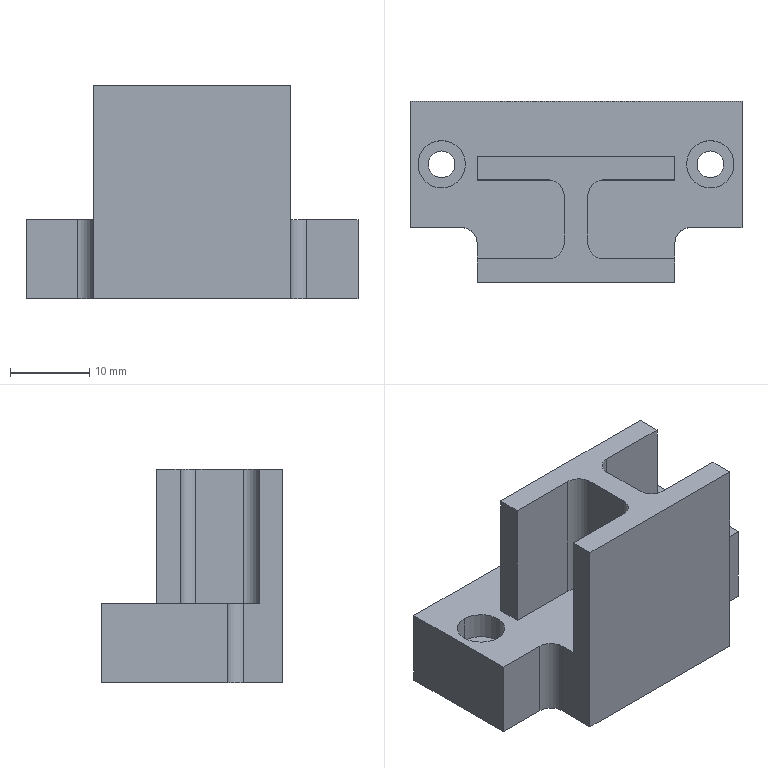Part | NX | 1 solid | 36 faces | box 42 x 23 x 27 mm | volume 11293 mm3 | plane 22 | cylinder 14 | commonest cylinder face diameters 4 x6 3.4 x4 6 x4
STEP:
#1=CARTESIAN_POINT('',(17.,6.5,-20.4));
#2=VERTEX_POINT('',#1);
#3=CARTESIAN_POINT('',(17.,0.5,-20.4));
#4=VERTEX_POINT('',#3);
#5=CARTESIAN_POINT('',(17.,3.5,-20.4));
#6=DIRECTION('',(0.,0.,1.));
#7=DIRECTION('',(0.,-1.,0.));
#8=AXIS2_PLACEMENT_3D('',#5,#6,#7);
#9=CIRCLE('',#8,3.);
#10=EDGE_CURVE('',#2,#4,#9,.T.);
#11=ORIENTED_EDGE('',*,*,#10,.F.);
#12=CARTESIAN_POINT('',(17.,6.5,-17.));
#13=VERTEX_POINT('',#12);
#14=CARTESIAN_POINT('',(17.,6.5,-17.));
#15=DIRECTION('',(0.,0.,1.));
#16=VECTOR('',#15,1000.);
#17=LINE('',#14,#16);
#18=EDGE_CURVE('',#13,#2,#17,.F.);
#19=ORIENTED_EDGE('',*,*,#18,.F.);
#20=CARTESIAN_POINT('',(17.,0.5,-17.));
#21=VERTEX_POINT('',#20);
#22=CARTESIAN_POINT('',(17.,3.5,-17.));
#23=DIRECTION('',(0.,0.,1.));
#24=DIRECTION('',(0.,-1.,0.));
#25=AXIS2_PLACEMENT_3D('',#22,#23,#24);
#26=CIRCLE('',#25,3.);
#27=EDGE_CURVE('',#13,#21,#26,.T.);
#28=ORIENTED_EDGE('',*,*,#27,.T.);
#29=CARTESIAN_POINT('',(17.,0.5,-17.));
#30=DIRECTION('',(0.,0.,1.));
#31=VECTOR('',#30,1000.);
#32=LINE('',#29,#31);
#33=EDGE_CURVE('',#21,#4,#32,.F.);
#34=ORIENTED_EDGE('',*,*,#33,.T.);
#35=EDGE_LOOP('',(#11,#19,#28,#34));
#36=FACE_BOUND('',#35,.T.);
#37=CARTESIAN_POINT('',(17.,3.5,-17.));
#38=DIRECTION('',(0.,0.,1.));
#39=DIRECTION('',(0.,1.,0.));
#40=AXIS2_PLACEMENT_3D('',#37,#38,#39);
#41=CYLINDRICAL_SURFACE('',#40,3.);
#42=ADVANCED_FACE('',(#36),#41,.F.);
#43=CARTESIAN_POINT('',(17.,5.2,-27.));
#44=VERTEX_POINT('',#43);
#45=CARTESIAN_POINT('',(17.,1.8,-27.));
#46=VERTEX_POINT('',#45);
#47=CARTESIAN_POINT('',(17.,3.5,-27.));
#48=DIRECTION('',(0.,0.,1.));
#49=DIRECTION('',(0.,-1.,0.));
#50=AXIS2_PLACEMENT_3D('',#47,#48,#49);
#51=CIRCLE('',#50,1.7);
#52=EDGE_CURVE('',#44,#46,#51,.T.);
#53=ORIENTED_EDGE('',*,*,#52,.F.);
#54=CARTESIAN_POINT('',(17.,5.2,-20.4));
#55=VERTEX_POINT('',#54);
#56=CARTESIAN_POINT('',(17.,5.2,-17.));
#57=DIRECTION('',(0.,0.,1.));
#58=VECTOR('',#57,1000.);
#59=LINE('',#56,#58);
#60=EDGE_CURVE('',#55,#44,#59,.F.);
#61=ORIENTED_EDGE('',*,*,#60,.F.);
#62=CARTESIAN_POINT('',(17.,1.8,-20.4));
#63=VERTEX_POINT('',#62);
#64=CARTESIAN_POINT('',(17.,3.5,-20.4));
#65=DIRECTION('',(0.,0.,1.));
#66=DIRECTION('',(0.,-1.,0.));
#67=AXIS2_PLACEMENT_3D('',#64,#65,#66);
#68=CIRCLE('',#67,1.7);
#69=EDGE_CURVE('',#55,#63,#68,.T.);
#70=ORIENTED_EDGE('',*,*,#69,.T.);
#71=CARTESIAN_POINT('',(17.,1.8,-17.));
#72=DIRECTION('',(0.,0.,1.));
#73=VECTOR('',#72,1000.);
#74=LINE('',#71,#73);
#75=EDGE_CURVE('',#63,#46,#74,.F.);
#76=ORIENTED_EDGE('',*,*,#75,.T.);
#77=EDGE_LOOP('',(#53,#61,#70,#76));
#78=FACE_BOUND('',#77,.T.);
#79=CARTESIAN_POINT('',(17.,3.5,-17.));
#80=DIRECTION('',(0.,0.,1.));
#81=DIRECTION('',(0.,1.,0.));
#82=AXIS2_PLACEMENT_3D('',#79,#80,#81);
#83=CYLINDRICAL_SURFACE('',#82,1.7);
#84=ADVANCED_FACE('',(#78),#83,.F.);
#85=CARTESIAN_POINT('',(-17.,6.5,-20.4));
#86=VERTEX_POINT('',#85);
#87=CARTESIAN_POINT('',(-17.,0.5,-20.4));
#88=VERTEX_POINT('',#87);
#89=CARTESIAN_POINT('',(-17.,3.5,-20.4));
#90=DIRECTION('',(0.,0.,1.));
#91=DIRECTION('',(0.,-1.,0.));
#92=AXIS2_PLACEMENT_3D('',#89,#90,#91);
#93=CIRCLE('',#92,3.);
#94=EDGE_CURVE('',#86,#88,#93,.T.);
#95=ORIENTED_EDGE('',*,*,#94,.F.);
#96=CARTESIAN_POINT('',(-17.,6.5,-17.));
#97=VERTEX_POINT('',#96);
#98=CARTESIAN_POINT('',(-17.,6.5,-17.));
#99=DIRECTION('',(0.,0.,1.));
#100=VECTOR('',#99,1000.);
#101=LINE('',#98,#100);
#102=EDGE_CURVE('',#97,#86,#101,.F.);
#103=ORIENTED_EDGE('',*,*,#102,.F.);
#104=CARTESIAN_POINT('',(-17.,0.5,-17.));
#105=VERTEX_POINT('',#104);
#106=CARTESIAN_POINT('',(-17.,3.5,-17.));
#107=DIRECTION('',(0.,0.,1.));
#108=DIRECTION('',(0.,-1.,0.));
#109=AXIS2_PLACEMENT_3D('',#106,#107,#108);
#110=CIRCLE('',#109,3.);
#111=EDGE_CURVE('',#97,#105,#110,.T.);
#112=ORIENTED_EDGE('',*,*,#111,.T.);
#113=CARTESIAN_POINT('',(-17.,0.5,-17.));
#114=DIRECTION('',(0.,0.,1.));
#115=VECTOR('',#114,1000.);
#116=LINE('',#113,#115);
#117=EDGE_CURVE('',#105,#88,#116,.F.);
#118=ORIENTED_EDGE('',*,*,#117,.T.);
#119=EDGE_LOOP('',(#95,#103,#112,#118));
#120=FACE_BOUND('',#119,.T.);
#121=CARTESIAN_POINT('',(-17.,3.5,-17.));
#122=DIRECTION('',(0.,0.,1.));
#123=DIRECTION('',(0.,1.,0.));
#124=AXIS2_PLACEMENT_3D('',#121,#122,#123);
#125=CYLINDRICAL_SURFACE('',#124,3.);
#126=ADVANCED_FACE('',(#120),#125,.F.);
#127=CARTESIAN_POINT('',(-17.,5.2,-27.));
#128=VERTEX_POINT('',#127);
#129=CARTESIAN_POINT('',(-17.,1.8,-27.));
#130=VERTEX_POINT('',#129);
#131=CARTESIAN_POINT('',(-17.,3.5,-27.));
#132=DIRECTION('',(0.,0.,1.));
#133=DIRECTION('',(0.,-1.,0.));
#134=AXIS2_PLACEMENT_3D('',#131,#132,#133);
#135=CIRCLE('',#134,1.7);
#136=EDGE_CURVE('',#128,#130,#135,.T.);
#137=ORIENTED_EDGE('',*,*,#136,.F.);
#138=CARTESIAN_POINT('',(-17.,5.2,-20.4));
#139=VERTEX_POINT('',#138);
#140=CARTESIAN_POINT('',(-17.,5.2,-17.));
#141=DIRECTION('',(0.,0.,1.));
#142=VECTOR('',#141,1000.);
#143=LINE('',#140,#142);
#144=EDGE_CURVE('',#139,#128,#143,.F.);
#145=ORIENTED_EDGE('',*,*,#144,.F.);
#146=CARTESIAN_POINT('',(-17.,1.8,-20.4));
#147=VERTEX_POINT('',#146);
#148=CARTESIAN_POINT('',(-17.,3.5,-20.4));
#149=DIRECTION('',(0.,0.,1.));
#150=DIRECTION('',(0.,-1.,0.));
#151=AXIS2_PLACEMENT_3D('',#148,#149,#150);
#152=CIRCLE('',#151,1.7);
#153=EDGE_CURVE('',#139,#147,#152,.T.);
#154=ORIENTED_EDGE('',*,*,#153,.T.);
#155=CARTESIAN_POINT('',(-17.,1.8,-17.));
#156=DIRECTION('',(0.,0.,1.));
#157=VECTOR('',#156,1000.);
#158=LINE('',#155,#157);
#159=EDGE_CURVE('',#147,#130,#158,.F.);
#160=ORIENTED_EDGE('',*,*,#159,.T.);
#161=EDGE_LOOP('',(#137,#145,#154,#160));
#162=FACE_BOUND('',#161,.T.);
#163=CARTESIAN_POINT('',(-17.,3.5,-17.));
#164=DIRECTION('',(0.,0.,1.));
#165=DIRECTION('',(0.,1.,0.));
#166=AXIS2_PLACEMENT_3D('',#163,#164,#165);
#167=CYLINDRICAL_SURFACE('',#166,1.7);
#168=ADVANCED_FACE('',(#162),#167,.F.);
#169=CARTESIAN_POINT('',(-17.,3.5,-17.));
#170=DIRECTION('',(0.,0.,1.));
#171=DIRECTION('',(0.,-1.,0.));
#172=AXIS2_PLACEMENT_3D('',#169,#170,#171);
#173=CIRCLE('',#172,3.);
#174=EDGE_CURVE('',#105,#97,#173,.T.);
#175=ORIENTED_EDGE('',*,*,#174,.F.);
#176=ORIENTED_EDGE('',*,*,#111,.F.);
#177=EDGE_LOOP('',(#175,#176));
#178=FACE_BOUND('',#177,.T.);
#179=CARTESIAN_POINT('',(17.,3.5,-17.));
#180=DIRECTION('',(0.,0.,1.));
#181=DIRECTION('',(0.,-1.,0.));
#182=AXIS2_PLACEMENT_3D('',#179,#180,#181);
#183=CIRCLE('',#182,3.);
#184=EDGE_CURVE('',#21,#13,#183,.T.);
#185=ORIENTED_EDGE('',*,*,#184,.F.);
#186=ORIENTED_EDGE('',*,*,#27,.F.);
#187=EDGE_LOOP('',(#185,#186));
#188=FACE_BOUND('',#187,.T.);
#189=CARTESIAN_POINT('',(-3.5,-8.5,-17.));
#190=VERTEX_POINT('',#189);
#191=CARTESIAN_POINT('',(-12.5,-8.5,-17.));
#192=VERTEX_POINT('',#191);
#193=CARTESIAN_POINT('',(-12.5,-8.5,-17.));
#194=DIRECTION('',(-1.,0.,0.));
#195=VECTOR('',#194,1000.);
#196=LINE('',#193,#195);
#197=EDGE_CURVE('',#190,#192,#196,.T.);
#198=ORIENTED_EDGE('',*,*,#197,.F.);
#199=CARTESIAN_POINT('',(-1.5,-6.5,-17.));
#200=VERTEX_POINT('',#199);
#201=CARTESIAN_POINT('',(-3.5,-6.5,-17.));
#202=DIRECTION('',(0.,0.,1.));
#203=DIRECTION('',(0.,1.,0.));
#204=AXIS2_PLACEMENT_3D('',#201,#202,#203);
#205=CIRCLE('',#204,2.);
#206=EDGE_CURVE('',#190,#200,#205,.T.);
#207=ORIENTED_EDGE('',*,*,#206,.T.);
#208=CARTESIAN_POINT('',(-1.5,-0.5,-17.));
#209=VERTEX_POINT('',#208);
#210=CARTESIAN_POINT('',(-1.5,1.5,-17.));
#211=DIRECTION('',(0.,-1.,0.));
#212=VECTOR('',#211,1000.);
#213=LINE('',#210,#212);
#214=EDGE_CURVE('',#209,#200,#213,.T.);
#215=ORIENTED_EDGE('',*,*,#214,.F.);
#216=CARTESIAN_POINT('',(-3.5,1.5,-17.));
#217=VERTEX_POINT('',#216);
#218=CARTESIAN_POINT('',(-3.5,-0.5,-17.));
#219=DIRECTION('',(0.,0.,1.));
#220=DIRECTION('',(0.,1.,0.));
#221=AXIS2_PLACEMENT_3D('',#218,#219,#220);
#222=CIRCLE('',#221,2.);
#223=EDGE_CURVE('',#209,#217,#222,.T.);
#224=ORIENTED_EDGE('',*,*,#223,.T.);
#225=CARTESIAN_POINT('',(-12.5,1.5,-17.));
#226=VERTEX_POINT('',#225);
#227=CARTESIAN_POINT('',(-12.5,1.5,-17.));
#228=DIRECTION('',(1.,0.,0.));
#229=VECTOR('',#228,1000.);
#230=LINE('',#227,#229);
#231=EDGE_CURVE('',#226,#217,#230,.T.);
#232=ORIENTED_EDGE('',*,*,#231,.F.);
#233=CARTESIAN_POINT('',(-12.5,4.5,-17.));
#234=VERTEX_POINT('',#233);
#235=CARTESIAN_POINT('',(-12.5,1.5,-17.));
#236=DIRECTION('',(0.,-1.,0.));
#237=VECTOR('',#236,1000.);
#238=LINE('',#235,#237);
#239=EDGE_CURVE('',#234,#226,#238,.T.);
#240=ORIENTED_EDGE('',*,*,#239,.F.);
#241=CARTESIAN_POINT('',(12.5,4.5,-17.));
#242=VERTEX_POINT('',#241);
#243=CARTESIAN_POINT('',(-12.5,4.5,-17.));
#244=DIRECTION('',(-1.,0.,0.));
#245=VECTOR('',#244,1000.);
#246=LINE('',#243,#245);
#247=EDGE_CURVE('',#242,#234,#246,.T.);
#248=ORIENTED_EDGE('',*,*,#247,.F.);
#249=CARTESIAN_POINT('',(12.5,1.5,-17.));
#250=VERTEX_POINT('',#249);
#251=CARTESIAN_POINT('',(12.5,1.5,-17.));
#252=DIRECTION('',(0.,1.,0.));
#253=VECTOR('',#252,1000.);
#254=LINE('',#251,#253);
#255=EDGE_CURVE('',#250,#242,#254,.T.);
#256=ORIENTED_EDGE('',*,*,#255,.F.);
#257=CARTESIAN_POINT('',(3.5,1.5,-17.));
#258=VERTEX_POINT('',#257);
#259=CARTESIAN_POINT('',(-12.5,1.5,-17.));
#260=DIRECTION('',(1.,0.,0.));
#261=VECTOR('',#260,1000.);
#262=LINE('',#259,#261);
#263=EDGE_CURVE('',#258,#250,#262,.T.);
#264=ORIENTED_EDGE('',*,*,#263,.F.);
#265=CARTESIAN_POINT('',(1.5,-0.5,-17.));
#266=VERTEX_POINT('',#265);
#267=CARTESIAN_POINT('',(3.5,-0.5,-17.));
#268=DIRECTION('',(0.,0.,1.));
#269=DIRECTION('',(0.,1.,0.));
#270=AXIS2_PLACEMENT_3D('',#267,#268,#269);
#271=CIRCLE('',#270,2.);
#272=EDGE_CURVE('',#258,#266,#271,.T.);
#273=ORIENTED_EDGE('',*,*,#272,.T.);
#274=CARTESIAN_POINT('',(1.5,-6.5,-17.));
#275=VERTEX_POINT('',#274);
#276=CARTESIAN_POINT('',(1.5,1.5,-17.));
#277=DIRECTION('',(0.,1.,0.));
#278=VECTOR('',#277,1000.);
#279=LINE('',#276,#278);
#280=EDGE_CURVE('',#275,#266,#279,.T.);
#281=ORIENTED_EDGE('',*,*,#280,.F.);
#282=CARTESIAN_POINT('',(3.5,-8.5,-17.));
#283=VERTEX_POINT('',#282);
#284=CARTESIAN_POINT('',(3.5,-6.5,-17.));
#285=DIRECTION('',(0.,0.,1.));
#286=DIRECTION('',(0.,1.,0.));
#287=AXIS2_PLACEMENT_3D('',#284,#285,#286);
#288=CIRCLE('',#287,2.);
#289=EDGE_CURVE('',#275,#283,#288,.T.);
#290=ORIENTED_EDGE('',*,*,#289,.T.);
#291=CARTESIAN_POINT('',(12.5,-8.5,-17.));
#292=VERTEX_POINT('',#291);
#293=CARTESIAN_POINT('',(-12.5,-8.5,-17.));
#294=DIRECTION('',(-1.,0.,0.));
#295=VECTOR('',#294,1000.);
#296=LINE('',#293,#295);
#297=EDGE_CURVE('',#292,#283,#296,.T.);
#298=ORIENTED_EDGE('',*,*,#297,.F.);
#299=CARTESIAN_POINT('',(12.5,-6.5,-17.));
#300=VERTEX_POINT('',#299);
#301=CARTESIAN_POINT('',(12.5,-11.5,-17.));
#302=DIRECTION('',(0.,1.,0.));
#303=VECTOR('',#302,1000.);
#304=LINE('',#301,#303);
#305=EDGE_CURVE('',#292,#300,#304,.T.);
#306=ORIENTED_EDGE('',*,*,#305,.T.);
#307=CARTESIAN_POINT('',(14.5,-4.5,-17.));
#308=VERTEX_POINT('',#307);
#309=CARTESIAN_POINT('',(14.5,-6.5,-17.));
#310=DIRECTION('',(0.,0.,-1.));
#311=DIRECTION('',(0.,1.,0.));
#312=AXIS2_PLACEMENT_3D('',#309,#310,#311);
#313=CIRCLE('',#312,2.);
#314=EDGE_CURVE('',#300,#308,#313,.T.);
#315=ORIENTED_EDGE('',*,*,#314,.T.);
#316=CARTESIAN_POINT('',(21.,-4.5,-17.));
#317=VERTEX_POINT('',#316);
#318=CARTESIAN_POINT('',(12.5,-4.5,-17.));
#319=DIRECTION('',(1.,0.,0.));
#320=VECTOR('',#319,1000.);
#321=LINE('',#318,#320);
#322=EDGE_CURVE('',#308,#317,#321,.T.);
#323=ORIENTED_EDGE('',*,*,#322,.T.);
#324=CARTESIAN_POINT('',(21.,11.5,-17.));
#325=VERTEX_POINT('',#324);
#326=CARTESIAN_POINT('',(21.,11.5,-17.));
#327=DIRECTION('',(0.,1.,0.));
#328=VECTOR('',#327,1000.);
#329=LINE('',#326,#328);
#330=EDGE_CURVE('',#317,#325,#329,.T.);
#331=ORIENTED_EDGE('',*,*,#330,.T.);
#332=CARTESIAN_POINT('',(-21.,11.5,-17.));
#333=VERTEX_POINT('',#332);
#334=CARTESIAN_POINT('',(-21.,11.5,-17.));
#335=DIRECTION('',(-1.,0.,0.));
#336=VECTOR('',#335,1000.);
#337=LINE('',#334,#336);
#338=EDGE_CURVE('',#325,#333,#337,.T.);
#339=ORIENTED_EDGE('',*,*,#338,.T.);
#340=CARTESIAN_POINT('',(-21.,-4.5,-17.));
#341=VERTEX_POINT('',#340);
#342=CARTESIAN_POINT('',(-21.,11.5,-17.));
#343=DIRECTION('',(0.,-1.,0.));
#344=VECTOR('',#343,1000.);
#345=LINE('',#342,#344);
#346=EDGE_CURVE('',#333,#341,#345,.T.);
#347=ORIENTED_EDGE('',*,*,#346,.T.);
#348=CARTESIAN_POINT('',(-14.5,-4.5,-17.));
#349=VERTEX_POINT('',#348);
#350=CARTESIAN_POINT('',(-21.,-4.5,-17.));
#351=DIRECTION('',(1.,0.,0.));
#352=VECTOR('',#351,1000.);
#353=LINE('',#350,#352);
#354=EDGE_CURVE('',#341,#349,#353,.T.);
#355=ORIENTED_EDGE('',*,*,#354,.T.);
#356=CARTESIAN_POINT('',(-12.5,-6.5,-17.));
#357=VERTEX_POINT('',#356);
#358=CARTESIAN_POINT('',(-14.5,-6.5,-17.));
#359=DIRECTION('',(0.,0.,-1.));
#360=DIRECTION('',(0.,1.,0.));
#361=AXIS2_PLACEMENT_3D('',#358,#359,#360);
#362=CIRCLE('',#361,2.);
#363=EDGE_CURVE('',#349,#357,#362,.T.);
#364=ORIENTED_EDGE('',*,*,#363,.T.);
#365=CARTESIAN_POINT('',(-12.5,-4.5,-17.));
#366=DIRECTION('',(0.,-1.,0.));
#367=VECTOR('',#366,1000.);
#368=LINE('',#365,#367);
#369=EDGE_CURVE('',#357,#192,#368,.T.);
#370=ORIENTED_EDGE('',*,*,#369,.T.);
#371=EDGE_LOOP('',(#198,#207,#215,#224,#232,#240,#248,#256,#264,#273,#281,#290,#298,#306,#315,#323,#331,#339,#347,#355,#364,#370));
#372=FACE_BOUND('',#371,.T.);
#373=CARTESIAN_POINT('',(0.,3.5,-17.));
#374=DIRECTION('',(0.,0.,-1.));
#375=DIRECTION('',(0.,-1.,0.));
#376=AXIS2_PLACEMENT_3D('',#373,#374,#375);
#377=PLANE('',#376);
#378=ADVANCED_FACE('',(#178,#188,#372),#377,.F.);
#379=CARTESIAN_POINT('',(-3.5,-8.5,0.));
#380=VERTEX_POINT('',#379);
#381=CARTESIAN_POINT('',(-12.5,-8.5,0.));
#382=VERTEX_POINT('',#381);
#383=CARTESIAN_POINT('',(-12.5,-8.5,0.));
#384=DIRECTION('',(-1.,0.,0.));
#385=VECTOR('',#384,1000.);
#386=LINE('',#383,#385);
#387=EDGE_CURVE('',#380,#382,#386,.T.);
#388=ORIENTED_EDGE('',*,*,#387,.F.);
#389=CARTESIAN_POINT('',(-3.5,-8.5,-17.));
#390=DIRECTION('',(0.,0.,-1.));
#391=VECTOR('',#390,1000.);
#392=LINE('',#389,#391);
#393=EDGE_CURVE('',#380,#190,#392,.T.);
#394=ORIENTED_EDGE('',*,*,#393,.T.);
#395=ORIENTED_EDGE('',*,*,#197,.T.);
#396=CARTESIAN_POINT('',(-12.5,-8.5,0.));
#397=DIRECTION('',(0.,0.,-1.));
#398=VECTOR('',#397,1000.);
#399=LINE('',#396,#398);
#400=EDGE_CURVE('',#382,#192,#399,.T.);
#401=ORIENTED_EDGE('',*,*,#400,.F.);
#402=EDGE_LOOP('',(#388,#394,#395,#401));
#403=FACE_BOUND('',#402,.T.);
#404=CARTESIAN_POINT('',(-12.5,-8.5,0.));
#405=DIRECTION('',(0.,-1.,0.));
#406=DIRECTION('',(-1.,0.,0.));
#407=AXIS2_PLACEMENT_3D('',#404,#405,#406);
#408=PLANE('',#407);
#409=ADVANCED_FACE('',(#403),#408,.F.);
#410=ORIENTED_EDGE('',*,*,#297,.T.);
#411=CARTESIAN_POINT('',(3.5,-8.5,0.));
#412=VERTEX_POINT('',#411);
#413=CARTESIAN_POINT('',(3.5,-8.5,0.));
#414=DIRECTION('',(0.,0.,1.));
#415=VECTOR('',#414,1000.);
#416=LINE('',#413,#415);
#417=EDGE_CURVE('',#283,#412,#416,.T.);
#418=ORIENTED_EDGE('',*,*,#417,.T.);
#419=CARTESIAN_POINT('',(12.5,-8.5,0.));
#420=VERTEX_POINT('',#419);
#421=CARTESIAN_POINT('',(-12.5,-8.5,0.));
#422=DIRECTION('',(-1.,0.,0.));
#423=VECTOR('',#422,1000.);
#424=LINE('',#421,#423);
#425=EDGE_CURVE('',#420,#412,#424,.T.);
#426=ORIENTED_EDGE('',*,*,#425,.F.);
#427=CARTESIAN_POINT('',(12.5,-8.5,0.));
#428=DIRECTION('',(0.,0.,-1.));
#429=VECTOR('',#428,1000.);
#430=LINE('',#427,#429);
#431=EDGE_CURVE('',#420,#292,#430,.T.);
#432=ORIENTED_EDGE('',*,*,#431,.T.);
#433=EDGE_LOOP('',(#410,#418,#426,#432));
#434=FACE_BOUND('',#433,.T.);
#435=CARTESIAN_POINT('',(-12.5,-8.5,0.));
#436=DIRECTION('',(0.,-1.,0.));
#437=DIRECTION('',(-1.,0.,0.));
#438=AXIS2_PLACEMENT_3D('',#435,#436,#437);
#439=PLANE('',#438);
#440=ADVANCED_FACE('',(#434),#439,.F.);
#441=ORIENTED_EDGE('',*,*,#231,.T.);
#442=CARTESIAN_POINT('',(-3.5,1.5,0.));
#443=VERTEX_POINT('',#442);
#444=CARTESIAN_POINT('',(-3.5,1.5,0.));
#445=DIRECTION('',(0.,0.,1.));
#446=VECTOR('',#445,1000.);
#447=LINE('',#444,#446);
#448=EDGE_CURVE('',#217,#443,#447,.T.);
#449=ORIENTED_EDGE('',*,*,#448,.T.);
#450=CARTESIAN_POINT('',(-12.5,1.5,0.));
#451=VERTEX_POINT('',#450);
#452=CARTESIAN_POINT('',(-12.5,1.5,0.));
#453=DIRECTION('',(1.,0.,0.));
#454=VECTOR('',#453,1000.);
#455=LINE('',#452,#454);
#456=EDGE_CURVE('',#451,#443,#455,.T.);
#457=ORIENTED_EDGE('',*,*,#456,.F.);
#458=CARTESIAN_POINT('',(-12.5,1.5,0.));
#459=DIRECTION('',(0.,0.,-1.));
#460=VECTOR('',#459,1000.);
#461=LINE('',#458,#460);
#462=EDGE_CURVE('',#451,#226,#461,.T.);
#463=ORIENTED_EDGE('',*,*,#462,.T.);
#464=EDGE_LOOP('',(#441,#449,#457,#463));
#465=FACE_BOUND('',#464,.T.);
#466=CARTESIAN_POINT('',(-12.5,1.5,0.));
#467=DIRECTION('',(0.,1.,0.));
#468=DIRECTION('',(1.,0.,0.));
#469=AXIS2_PLACEMENT_3D('',#466,#467,#468);
#470=PLANE('',#469);
#471=ADVANCED_FACE('',(#465),#470,.F.);
#472=CARTESIAN_POINT('',(3.5,1.5,0.));
#473=VERTEX_POINT('',#472);
#474=CARTESIAN_POINT('',(12.5,1.5,0.));
#475=VERTEX_POINT('',#474);
#476=CARTESIAN_POINT('',(-12.5,1.5,0.));
#477=DIRECTION('',(1.,0.,0.));
#478=VECTOR('',#477,1000.);
#479=LINE('',#476,#478);
#480=EDGE_CURVE('',#473,#475,#479,.T.);
#481=ORIENTED_EDGE('',*,*,#480,.F.);
#482=CARTESIAN_POINT('',(3.5,1.5,-17.));
#483=DIRECTION('',(0.,0.,-1.));
#484=VECTOR('',#483,1000.);
#485=LINE('',#482,#484);
#486=EDGE_CURVE('',#473,#258,#485,.T.);
#487=ORIENTED_EDGE('',*,*,#486,.T.);
#488=ORIENTED_EDGE('',*,*,#263,.T.);
#489=CARTESIAN_POINT('',(12.5,1.5,0.));
#490=DIRECTION('',(0.,0.,-1.));
#491=VECTOR('',#490,1000.);
#492=LINE('',#489,#491);
#493=EDGE_CURVE('',#475,#250,#492,.T.);
#494=ORIENTED_EDGE('',*,*,#493,.F.);
#495=EDGE_LOOP('',(#481,#487,#488,#494));
#496=FACE_BOUND('',#495,.T.);
#497=CARTESIAN_POINT('',(-12.5,1.5,0.));
#498=DIRECTION('',(0.,1.,0.));
#499=DIRECTION('',(1.,0.,0.));
#500=AXIS2_PLACEMENT_3D('',#497,#498,#499);
#501=PLANE('',#500);
#502=ADVANCED_FACE('',(#496),#501,.F.);
#503=ORIENTED_EDGE('',*,*,#322,.F.);
#504=CARTESIAN_POINT('',(14.5,-4.5,-27.));
#505=VERTEX_POINT('',#504);
#506=CARTESIAN_POINT('',(14.5,-4.5,-27.));
#507=DIRECTION('',(0.,0.,-1.));
#508=VECTOR('',#507,1000.);
#509=LINE('',#506,#508);
#510=EDGE_CURVE('',#308,#505,#509,.T.);
#511=ORIENTED_EDGE('',*,*,#510,.T.);
#512=CARTESIAN_POINT('',(21.,-4.5,-27.));
#513=VERTEX_POINT('',#512);
#514=CARTESIAN_POINT('',(12.5,-4.5,-27.));
#515=DIRECTION('',(1.,0.,0.));
#516=VECTOR('',#515,1000.);
#517=LINE('',#514,#516);
#518=EDGE_CURVE('',#505,#513,#517,.T.);
#519=ORIENTED_EDGE('',*,*,#518,.T.);
#520=CARTESIAN_POINT('',(21.,-4.5,-17.));
#521=DIRECTION('',(0.,0.,-1.));
#522=VECTOR('',#521,1000.);
#523=LINE('',#520,#522);
#524=EDGE_CURVE('',#317,#513,#523,.T.);
#525=ORIENTED_EDGE('',*,*,#524,.F.);
#526=EDGE_LOOP('',(#503,#511,#519,#525));
#527=FACE_BOUND('',#526,.T.);
#528=CARTESIAN_POINT('',(12.5,-4.5,-17.));
#529=DIRECTION('',(0.,1.,0.));
#530=DIRECTION('',(1.,0.,0.));
#531=AXIS2_PLACEMENT_3D('',#528,#529,#530);
#532=PLANE('',#531);
#533=ADVANCED_FACE('',(#527),#532,.F.);
#534=CARTESIAN_POINT('',(21.,11.5,-27.));
#535=VERTEX_POINT('',#534);
#536=CARTESIAN_POINT('',(21.,11.5,-27.));
#537=DIRECTION('',(0.,1.,0.));
#538=VECTOR('',#537,1000.);
#539=LINE('',#536,#538);
#540=EDGE_CURVE('',#513,#535,#539,.T.);
#541=ORIENTED_EDGE('',*,*,#540,.T.);
#542=CARTESIAN_POINT('',(21.,11.5,-17.));
#543=DIRECTION('',(0.,0.,-1.));
#544=VECTOR('',#543,1000.);
#545=LINE('',#542,#544);
#546=EDGE_CURVE('',#325,#535,#545,.T.);
#547=ORIENTED_EDGE('',*,*,#546,.F.);
#548=ORIENTED_EDGE('',*,*,#330,.F.);
#549=ORIENTED_EDGE('',*,*,#524,.T.);
#550=EDGE_LOOP('',(#541,#547,#548,#549));
#551=FACE_BOUND('',#550,.T.);
#552=CARTESIAN_POINT('',(21.,11.5,-17.));
#553=DIRECTION('',(-1.,0.,0.));
#554=DIRECTION('',(0.,1.,0.));
#555=AXIS2_PLACEMENT_3D('',#552,#553,#554);
#556=PLANE('',#555);
#557=ADVANCED_FACE('',(#551),#556,.F.);
#558=CARTESIAN_POINT('',(-21.,11.5,-27.));
#559=VERTEX_POINT('',#558);
#560=CARTESIAN_POINT('',(-21.,11.5,-27.));
#561=DIRECTION('',(-1.,0.,0.));
#562=VECTOR('',#561,1000.);
#563=LINE('',#560,#562);
#564=EDGE_CURVE('',#535,#559,#563,.T.);
#565=ORIENTED_EDGE('',*,*,#564,.T.);
#566=CARTESIAN_POINT('',(-21.,11.5,-17.));
#567=DIRECTION('',(0.,0.,-1.));
#568=VECTOR('',#567,1000.);
#569=LINE('',#566,#568);
#570=EDGE_CURVE('',#333,#559,#569,.T.);
#571=ORIENTED_EDGE('',*,*,#570,.F.);
#572=ORIENTED_EDGE('',*,*,#338,.F.);
#573=ORIENTED_EDGE('',*,*,#546,.T.);
#574=EDGE_LOOP('',(#565,#571,#572,#573));
#575=FACE_BOUND('',#574,.T.);
#576=CARTESIAN_POINT('',(-21.,11.5,-17.));
#577=DIRECTION('',(0.,-1.,0.));
#578=DIRECTION('',(-1.,0.,0.));
#579=AXIS2_PLACEMENT_3D('',#576,#577,#578);
#580=PLANE('',#579);
#581=ADVANCED_FACE('',(#575),#580,.F.);
#582=CARTESIAN_POINT('',(-21.,-4.5,-27.));
#583=VERTEX_POINT('',#582);
#584=CARTESIAN_POINT('',(-21.,11.5,-27.));
#585=DIRECTION('',(0.,-1.,0.));
#586=VECTOR('',#585,1000.);
#587=LINE('',#584,#586);
#588=EDGE_CURVE('',#559,#583,#587,.T.);
#589=ORIENTED_EDGE('',*,*,#588,.T.);
#590=CARTESIAN_POINT('',(-21.,-4.5,-17.));
#591=DIRECTION('',(0.,0.,-1.));
#592=VECTOR('',#591,1000.);
#593=LINE('',#590,#592);
#594=EDGE_CURVE('',#341,#583,#593,.T.);
#595=ORIENTED_EDGE('',*,*,#594,.F.);
#596=ORIENTED_EDGE('',*,*,#346,.F.);
#597=ORIENTED_EDGE('',*,*,#570,.T.);
#598=EDGE_LOOP('',(#589,#595,#596,#597));
#599=FACE_BOUND('',#598,.T.);
#600=CARTESIAN_POINT('',(-21.,11.5,-17.));
#601=DIRECTION('',(1.,0.,0.));
#602=DIRECTION('',(0.,-1.,0.));
#603=AXIS2_PLACEMENT_3D('',#600,#601,#602);
#604=PLANE('',#603);
#605=ADVANCED_FACE('',(#599),#604,.F.);
#606=CARTESIAN_POINT('',(-14.5,-4.5,-27.));
#607=VERTEX_POINT('',#606);
#608=CARTESIAN_POINT('',(-21.,-4.5,-27.));
#609=DIRECTION('',(1.,0.,0.));
#610=VECTOR('',#609,1000.);
#611=LINE('',#608,#610);
#612=EDGE_CURVE('',#583,#607,#611,.T.);
#613=ORIENTED_EDGE('',*,*,#612,.T.);
#614=CARTESIAN_POINT('',(-14.5,-4.5,-17.));
#615=DIRECTION('',(0.,0.,1.));
#616=VECTOR('',#615,1000.);
#617=LINE('',#614,#616);
#618=EDGE_CURVE('',#607,#349,#617,.T.);
#619=ORIENTED_EDGE('',*,*,#618,.T.);
#620=ORIENTED_EDGE('',*,*,#354,.F.);
#621=ORIENTED_EDGE('',*,*,#594,.T.);
#622=EDGE_LOOP('',(#613,#619,#620,#621));
#623=FACE_BOUND('',#622,.T.);
#624=CARTESIAN_POINT('',(-21.,-4.5,-17.));
#625=DIRECTION('',(0.,1.,0.));
#626=DIRECTION('',(1.,0.,0.));
#627=AXIS2_PLACEMENT_3D('',#624,#625,#626);
#628=PLANE('',#627);
#629=ADVANCED_FACE('',(#623),#628,.F.);
#630=ORIENTED_EDGE('',*,*,#369,.F.);
#631=CARTESIAN_POINT('',(-12.5,-6.5,-27.));
#632=VERTEX_POINT('',#631);
#633=CARTESIAN_POINT('',(-12.5,-6.5,-27.));
#634=DIRECTION('',(0.,0.,-1.));
#635=VECTOR('',#634,1000.);
#636=LINE('',#633,#635);
#637=EDGE_CURVE('',#357,#632,#636,.T.);
#638=ORIENTED_EDGE('',*,*,#637,.T.);
#639=CARTESIAN_POINT('',(-12.5,-11.5,-27.));
#640=VERTEX_POINT('',#639);
#641=CARTESIAN_POINT('',(-12.5,-4.5,-27.));
#642=DIRECTION('',(0.,-1.,0.));
#643=VECTOR('',#642,1000.);
#644=LINE('',#641,#643);
#645=EDGE_CURVE('',#632,#640,#644,.T.);
#646=ORIENTED_EDGE('',*,*,#645,.T.);
#647=CARTESIAN_POINT('',(-12.5,-11.5,0.));
#648=VERTEX_POINT('',#647);
#649=CARTESIAN_POINT('',(-12.5,-11.5,-17.));
#650=DIRECTION('',(0.,0.,-1.));
#651=VECTOR('',#650,1000.);
#652=LINE('',#649,#651);
#653=EDGE_CURVE('',#648,#640,#652,.T.);
#654=ORIENTED_EDGE('',*,*,#653,.F.);
#655=CARTESIAN_POINT('',(-12.5,-11.5,0.));
#656=DIRECTION('',(0.,-1.,0.));
#657=VECTOR('',#656,1000.);
#658=LINE('',#655,#657);
#659=EDGE_CURVE('',#382,#648,#658,.T.);
#660=ORIENTED_EDGE('',*,*,#659,.F.);
#661=ORIENTED_EDGE('',*,*,#400,.T.);
#662=EDGE_LOOP('',(#630,#638,#646,#654,#660,#661));
#663=FACE_BOUND('',#662,.T.);
#664=CARTESIAN_POINT('',(-12.5,-4.5,-17.));
#665=DIRECTION('',(1.,0.,0.));
#666=DIRECTION('',(0.,-1.,0.));
#667=AXIS2_PLACEMENT_3D('',#664,#665,#666);
#668=PLANE('',#667);
#669=ADVANCED_FACE('',(#663),#668,.F.);
#670=CARTESIAN_POINT('',(12.5,-11.5,-27.));
#671=VERTEX_POINT('',#670);
#672=CARTESIAN_POINT('',(-12.5,-11.5,-27.));
#673=DIRECTION('',(1.,0.,0.));
#674=VECTOR('',#673,1000.);
#675=LINE('',#672,#674);
#676=EDGE_CURVE('',#640,#671,#675,.T.);
#677=ORIENTED_EDGE('',*,*,#676,.T.);
#678=CARTESIAN_POINT('',(12.5,-11.5,0.));
#679=VERTEX_POINT('',#678);
#680=CARTESIAN_POINT('',(12.5,-11.5,-17.));
#681=DIRECTION('',(0.,0.,-1.));
#682=VECTOR('',#681,1000.);
#683=LINE('',#680,#682);
#684=EDGE_CURVE('',#679,#671,#683,.T.);
#685=ORIENTED_EDGE('',*,*,#684,.F.);
#686=CARTESIAN_POINT('',(-12.5,-11.5,0.));
#687=DIRECTION('',(1.,0.,0.));
#688=VECTOR('',#687,1000.);
#689=LINE('',#686,#688);
#690=EDGE_CURVE('',#648,#679,#689,.T.);
#691=ORIENTED_EDGE('',*,*,#690,.F.);
#692=ORIENTED_EDGE('',*,*,#653,.T.);
#693=EDGE_LOOP('',(#677,#685,#691,#692));
#694=FACE_BOUND('',#693,.T.);
#695=CARTESIAN_POINT('',(-12.5,-11.5,-17.));
#696=DIRECTION('',(0.,1.,0.));
#697=DIRECTION('',(1.,0.,0.));
#698=AXIS2_PLACEMENT_3D('',#695,#696,#697);
#699=PLANE('',#698);
#700=ADVANCED_FACE('',(#694),#699,.F.);
#701=CARTESIAN_POINT('',(12.5,-6.5,-27.));
#702=VERTEX_POINT('',#701);
#703=CARTESIAN_POINT('',(12.5,-11.5,-27.));
#704=DIRECTION('',(0.,1.,0.));
#705=VECTOR('',#704,1000.);
#706=LINE('',#703,#705);
#707=EDGE_CURVE('',#671,#702,#706,.T.);
#708=ORIENTED_EDGE('',*,*,#707,.T.);
#709=CARTESIAN_POINT('',(12.5,-6.5,-17.));
#710=DIRECTION('',(0.,0.,1.));
#711=VECTOR('',#710,1000.);
#712=LINE('',#709,#711);
#713=EDGE_CURVE('',#702,#300,#712,.T.);
#714=ORIENTED_EDGE('',*,*,#713,.T.);
#715=ORIENTED_EDGE('',*,*,#305,.F.);
#716=ORIENTED_EDGE('',*,*,#431,.F.);
#717=CARTESIAN_POINT('',(12.5,-11.5,0.));
#718=DIRECTION('',(0.,1.,0.));
#719=VECTOR('',#718,1000.);
#720=LINE('',#717,#719);
#721=EDGE_CURVE('',#679,#420,#720,.T.);
#722=ORIENTED_EDGE('',*,*,#721,.F.);
#723=ORIENTED_EDGE('',*,*,#684,.T.);
#724=EDGE_LOOP('',(#708,#714,#715,#716,#722,#723));
#725=FACE_BOUND('',#724,.T.);
#726=CARTESIAN_POINT('',(12.5,-11.5,-17.));
#727=DIRECTION('',(-1.,0.,0.));
#728=DIRECTION('',(0.,1.,0.));
#729=AXIS2_PLACEMENT_3D('',#726,#727,#728);
#730=PLANE('',#729);
#731=ADVANCED_FACE('',(#725),#730,.F.);
#732=CARTESIAN_POINT('',(17.,3.5,-27.));
#733=DIRECTION('',(0.,0.,1.));
#734=DIRECTION('',(0.,-1.,0.));
#735=AXIS2_PLACEMENT_3D('',#732,#733,#734);
#736=CIRCLE('',#735,1.7);
#737=EDGE_CURVE('',#46,#44,#736,.T.);
#738=ORIENTED_EDGE('',*,*,#737,.T.);
#739=ORIENTED_EDGE('',*,*,#52,.T.);
#740=EDGE_LOOP('',(#738,#739));
#741=FACE_BOUND('',#740,.T.);
#742=CARTESIAN_POINT('',(-17.,3.5,-27.));
#743=DIRECTION('',(0.,0.,1.));
#744=DIRECTION('',(0.,-1.,0.));
#745=AXIS2_PLACEMENT_3D('',#742,#743,#744);
#746=CIRCLE('',#745,1.7);
#747=EDGE_CURVE('',#130,#128,#746,.T.);
#748=ORIENTED_EDGE('',*,*,#747,.T.);
#749=ORIENTED_EDGE('',*,*,#136,.T.);
#750=EDGE_LOOP('',(#748,#749));
#751=FACE_BOUND('',#750,.T.);
#752=ORIENTED_EDGE('',*,*,#518,.F.);
#753=CARTESIAN_POINT('',(14.5,-6.5,-27.));
#754=DIRECTION('',(0.,0.,1.));
#755=DIRECTION('',(0.,1.,0.));
#756=AXIS2_PLACEMENT_3D('',#753,#754,#755);
#757=CIRCLE('',#756,2.);
#758=EDGE_CURVE('',#505,#702,#757,.T.);
#759=ORIENTED_EDGE('',*,*,#758,.T.);
#760=ORIENTED_EDGE('',*,*,#707,.F.);
#761=ORIENTED_EDGE('',*,*,#676,.F.);
#762=ORIENTED_EDGE('',*,*,#645,.F.);
#763=CARTESIAN_POINT('',(-14.5,-6.5,-27.));
#764=DIRECTION('',(0.,0.,1.));
#765=DIRECTION('',(0.,1.,0.));
#766=AXIS2_PLACEMENT_3D('',#763,#764,#765);
#767=CIRCLE('',#766,2.);
#768=EDGE_CURVE('',#632,#607,#767,.T.);
#769=ORIENTED_EDGE('',*,*,#768,.T.);
#770=ORIENTED_EDGE('',*,*,#612,.F.);
#771=ORIENTED_EDGE('',*,*,#588,.F.);
#772=ORIENTED_EDGE('',*,*,#564,.F.);
#773=ORIENTED_EDGE('',*,*,#540,.F.);
#774=EDGE_LOOP('',(#752,#759,#760,#761,#762,#769,#770,#771,#772,#773));
#775=FACE_BOUND('',#774,.T.);
#776=CARTESIAN_POINT('',(0.,3.5,-27.));
#777=DIRECTION('',(0.,0.,-1.));
#778=DIRECTION('',(0.,-1.,0.));
#779=AXIS2_PLACEMENT_3D('',#776,#777,#778);
#780=PLANE('',#779);
#781=ADVANCED_FACE('',(#741,#751,#775),#780,.T.);
#782=ORIENTED_EDGE('',*,*,#144,.T.);
#783=ORIENTED_EDGE('',*,*,#747,.F.);
#784=ORIENTED_EDGE('',*,*,#159,.F.);
#785=CARTESIAN_POINT('',(-17.,3.5,-20.4));
#786=DIRECTION('',(0.,0.,1.));
#787=DIRECTION('',(0.,-1.,0.));
#788=AXIS2_PLACEMENT_3D('',#785,#786,#787);
#789=CIRCLE('',#788,1.7);
#790=EDGE_CURVE('',#147,#139,#789,.T.);
#791=ORIENTED_EDGE('',*,*,#790,.T.);
#792=EDGE_LOOP('',(#782,#783,#784,#791));
#793=FACE_BOUND('',#792,.T.);
#794=CARTESIAN_POINT('',(-17.,3.5,-17.));
#795=DIRECTION('',(0.,0.,1.));
#796=DIRECTION('',(0.,1.,0.));
#797=AXIS2_PLACEMENT_3D('',#794,#795,#796);
#798=CYLINDRICAL_SURFACE('',#797,1.7);
#799=ADVANCED_FACE('',(#793),#798,.F.);
#800=ORIENTED_EDGE('',*,*,#790,.F.);
#801=ORIENTED_EDGE('',*,*,#153,.F.);
#802=EDGE_LOOP('',(#800,#801));
#803=FACE_BOUND('',#802,.T.);
#804=CARTESIAN_POINT('',(-17.,3.5,-20.4));
#805=DIRECTION('',(0.,0.,1.));
#806=DIRECTION('',(0.,-1.,0.));
#807=AXIS2_PLACEMENT_3D('',#804,#805,#806);
#808=CIRCLE('',#807,3.);
#809=EDGE_CURVE('',#88,#86,#808,.T.);
#810=ORIENTED_EDGE('',*,*,#809,.T.);
#811=ORIENTED_EDGE('',*,*,#94,.T.);
#812=EDGE_LOOP('',(#810,#811));
#813=FACE_BOUND('',#812,.T.);
#814=CARTESIAN_POINT('',(-15.3,3.5,-20.4));
#815=DIRECTION('',(0.,0.,-1.));
#816=DIRECTION('',(0.,-1.,0.));
#817=AXIS2_PLACEMENT_3D('',#814,#815,#816);
#818=PLANE('',#817);
#819=ADVANCED_FACE('',(#803,#813),#818,.F.);
#820=ORIENTED_EDGE('',*,*,#102,.T.);
#821=ORIENTED_EDGE('',*,*,#809,.F.);
#822=ORIENTED_EDGE('',*,*,#117,.F.);
#823=ORIENTED_EDGE('',*,*,#174,.T.);
#824=EDGE_LOOP('',(#820,#821,#822,#823));
#825=FACE_BOUND('',#824,.T.);
#826=CARTESIAN_POINT('',(-17.,3.5,-17.));
#827=DIRECTION('',(0.,0.,1.));
#828=DIRECTION('',(0.,1.,0.));
#829=AXIS2_PLACEMENT_3D('',#826,#827,#828);
#830=CYLINDRICAL_SURFACE('',#829,3.);
#831=ADVANCED_FACE('',(#825),#830,.F.);
#832=ORIENTED_EDGE('',*,*,#60,.T.);
#833=ORIENTED_EDGE('',*,*,#737,.F.);
#834=ORIENTED_EDGE('',*,*,#75,.F.);
#835=CARTESIAN_POINT('',(17.,3.5,-20.4));
#836=DIRECTION('',(0.,0.,1.));
#837=DIRECTION('',(0.,-1.,0.));
#838=AXIS2_PLACEMENT_3D('',#835,#836,#837);
#839=CIRCLE('',#838,1.7);
#840=EDGE_CURVE('',#63,#55,#839,.T.);
#841=ORIENTED_EDGE('',*,*,#840,.T.);
#842=EDGE_LOOP('',(#832,#833,#834,#841));
#843=FACE_BOUND('',#842,.T.);
#844=CARTESIAN_POINT('',(17.,3.5,-17.));
#845=DIRECTION('',(0.,0.,1.));
#846=DIRECTION('',(0.,1.,0.));
#847=AXIS2_PLACEMENT_3D('',#844,#845,#846);
#848=CYLINDRICAL_SURFACE('',#847,1.7);
#849=ADVANCED_FACE('',(#843),#848,.F.);
#850=ORIENTED_EDGE('',*,*,#840,.F.);
#851=ORIENTED_EDGE('',*,*,#69,.F.);
#852=EDGE_LOOP('',(#850,#851));
#853=FACE_BOUND('',#852,.T.);
#854=CARTESIAN_POINT('',(17.,3.5,-20.4));
#855=DIRECTION('',(0.,0.,1.));
#856=DIRECTION('',(0.,-1.,0.));
#857=AXIS2_PLACEMENT_3D('',#854,#855,#856);
#858=CIRCLE('',#857,3.);
#859=EDGE_CURVE('',#4,#2,#858,.T.);
#860=ORIENTED_EDGE('',*,*,#859,.T.);
#861=ORIENTED_EDGE('',*,*,#10,.T.);
#862=EDGE_LOOP('',(#860,#861));
#863=FACE_BOUND('',#862,.T.);
#864=CARTESIAN_POINT('',(18.7,3.5,-20.4));
#865=DIRECTION('',(0.,0.,-1.));
#866=DIRECTION('',(0.,-1.,0.));
#867=AXIS2_PLACEMENT_3D('',#864,#865,#866);
#868=PLANE('',#867);
#869=ADVANCED_FACE('',(#853,#863),#868,.F.);
#870=ORIENTED_EDGE('',*,*,#18,.T.);
#871=ORIENTED_EDGE('',*,*,#859,.F.);
#872=ORIENTED_EDGE('',*,*,#33,.F.);
#873=ORIENTED_EDGE('',*,*,#184,.T.);
#874=EDGE_LOOP('',(#870,#871,#872,#873));
#875=FACE_BOUND('',#874,.T.);
#876=CARTESIAN_POINT('',(17.,3.5,-17.));
#877=DIRECTION('',(0.,0.,1.));
#878=DIRECTION('',(0.,1.,0.));
#879=AXIS2_PLACEMENT_3D('',#876,#877,#878);
#880=CYLINDRICAL_SURFACE('',#879,3.);
#881=ADVANCED_FACE('',(#875),#880,.F.);
#882=ORIENTED_EDGE('',*,*,#659,.T.);
#883=ORIENTED_EDGE('',*,*,#690,.T.);
#884=ORIENTED_EDGE('',*,*,#721,.T.);
#885=ORIENTED_EDGE('',*,*,#425,.T.);
#886=CARTESIAN_POINT('',(1.5,-6.5,0.));
#887=VERTEX_POINT('',#886);
#888=CARTESIAN_POINT('',(3.5,-6.5,0.));
#889=DIRECTION('',(0.,0.,-1.));
#890=DIRECTION('',(0.,1.,0.));
#891=AXIS2_PLACEMENT_3D('',#888,#889,#890);
#892=CIRCLE('',#891,2.);
#893=EDGE_CURVE('',#412,#887,#892,.T.);
#894=ORIENTED_EDGE('',*,*,#893,.T.);
#895=CARTESIAN_POINT('',(1.5,-0.5,0.));
#896=VERTEX_POINT('',#895);
#897=CARTESIAN_POINT('',(1.5,1.5,0.));
#898=DIRECTION('',(0.,-1.,0.));
#899=VECTOR('',#898,1000.);
#900=LINE('',#897,#899);
#901=EDGE_CURVE('',#896,#887,#900,.T.);
#902=ORIENTED_EDGE('',*,*,#901,.F.);
#903=CARTESIAN_POINT('',(3.5,-0.5,0.));
#904=DIRECTION('',(0.,0.,-1.));
#905=DIRECTION('',(0.,1.,0.));
#906=AXIS2_PLACEMENT_3D('',#903,#904,#905);
#907=CIRCLE('',#906,2.);
#908=EDGE_CURVE('',#896,#473,#907,.T.);
#909=ORIENTED_EDGE('',*,*,#908,.T.);
#910=ORIENTED_EDGE('',*,*,#480,.T.);
#911=CARTESIAN_POINT('',(12.5,4.5,0.));
#912=VERTEX_POINT('',#911);
#913=CARTESIAN_POINT('',(12.5,1.5,0.));
#914=DIRECTION('',(0.,1.,0.));
#915=VECTOR('',#914,1000.);
#916=LINE('',#913,#915);
#917=EDGE_CURVE('',#475,#912,#916,.T.);
#918=ORIENTED_EDGE('',*,*,#917,.T.);
#919=CARTESIAN_POINT('',(-12.5,4.5,0.));
#920=VERTEX_POINT('',#919);
#921=CARTESIAN_POINT('',(-12.5,4.5,0.));
#922=DIRECTION('',(-1.,0.,0.));
#923=VECTOR('',#922,1000.);
#924=LINE('',#921,#923);
#925=EDGE_CURVE('',#912,#920,#924,.T.);
#926=ORIENTED_EDGE('',*,*,#925,.T.);
#927=CARTESIAN_POINT('',(-12.5,1.5,0.));
#928=DIRECTION('',(0.,-1.,0.));
#929=VECTOR('',#928,1000.);
#930=LINE('',#927,#929);
#931=EDGE_CURVE('',#920,#451,#930,.T.);
#932=ORIENTED_EDGE('',*,*,#931,.T.);
#933=ORIENTED_EDGE('',*,*,#456,.T.);
#934=CARTESIAN_POINT('',(-1.5,-0.5,0.));
#935=VERTEX_POINT('',#934);
#936=CARTESIAN_POINT('',(-3.5,-0.5,0.));
#937=DIRECTION('',(0.,0.,-1.));
#938=DIRECTION('',(0.,1.,0.));
#939=AXIS2_PLACEMENT_3D('',#936,#937,#938);
#940=CIRCLE('',#939,2.);
#941=EDGE_CURVE('',#443,#935,#940,.T.);
#942=ORIENTED_EDGE('',*,*,#941,.T.);
#943=CARTESIAN_POINT('',(-1.5,-6.5,0.));
#944=VERTEX_POINT('',#943);
#945=CARTESIAN_POINT('',(-1.5,1.5,0.));
#946=DIRECTION('',(0.,1.,0.));
#947=VECTOR('',#946,1000.);
#948=LINE('',#945,#947);
#949=EDGE_CURVE('',#944,#935,#948,.T.);
#950=ORIENTED_EDGE('',*,*,#949,.F.);
#951=CARTESIAN_POINT('',(-3.5,-6.5,0.));
#952=DIRECTION('',(0.,0.,-1.));
#953=DIRECTION('',(0.,1.,0.));
#954=AXIS2_PLACEMENT_3D('',#951,#952,#953);
#955=CIRCLE('',#954,2.);
#956=EDGE_CURVE('',#944,#380,#955,.T.);
#957=ORIENTED_EDGE('',*,*,#956,.T.);
#958=ORIENTED_EDGE('',*,*,#387,.T.);
#959=EDGE_LOOP('',(#882,#883,#884,#885,#894,#902,#909,#910,#918,#926,#932,#933,#942,#950,#957,#958));
#960=FACE_BOUND('',#959,.T.);
#961=CARTESIAN_POINT('',(0.,3.5,0.));
#962=DIRECTION('',(0.,0.,-1.));
#963=DIRECTION('',(0.,-1.,0.));
#964=AXIS2_PLACEMENT_3D('',#961,#962,#963);
#965=PLANE('',#964);
#966=ADVANCED_FACE('',(#960),#965,.F.);
#967=ORIENTED_EDGE('',*,*,#239,.T.);
#968=ORIENTED_EDGE('',*,*,#462,.F.);
#969=ORIENTED_EDGE('',*,*,#931,.F.);
#970=CARTESIAN_POINT('',(-12.5,4.5,0.));
#971=DIRECTION('',(0.,0.,-1.));
#972=VECTOR('',#971,1000.);
#973=LINE('',#970,#972);
#974=EDGE_CURVE('',#920,#234,#973,.T.);
#975=ORIENTED_EDGE('',*,*,#974,.T.);
#976=EDGE_LOOP('',(#967,#968,#969,#975));
#977=FACE_BOUND('',#976,.T.);
#978=CARTESIAN_POINT('',(-12.5,1.5,0.));
#979=DIRECTION('',(1.,0.,0.));
#980=DIRECTION('',(0.,-1.,0.));
#981=AXIS2_PLACEMENT_3D('',#978,#979,#980);
#982=PLANE('',#981);
#983=ADVANCED_FACE('',(#977),#982,.F.);
#984=ORIENTED_EDGE('',*,*,#255,.T.);
#985=CARTESIAN_POINT('',(12.5,4.5,0.));
#986=DIRECTION('',(0.,0.,-1.));
#987=VECTOR('',#986,1000.);
#988=LINE('',#985,#987);
#989=EDGE_CURVE('',#912,#242,#988,.T.);
#990=ORIENTED_EDGE('',*,*,#989,.F.);
#991=ORIENTED_EDGE('',*,*,#917,.F.);
#992=ORIENTED_EDGE('',*,*,#493,.T.);
#993=EDGE_LOOP('',(#984,#990,#991,#992));
#994=FACE_BOUND('',#993,.T.);
#995=CARTESIAN_POINT('',(12.5,1.5,0.));
#996=DIRECTION('',(-1.,0.,0.));
#997=DIRECTION('',(0.,1.,0.));
#998=AXIS2_PLACEMENT_3D('',#995,#996,#997);
#999=PLANE('',#998);
#1000=ADVANCED_FACE('',(#994),#999,.F.);
#1001=ORIENTED_EDGE('',*,*,#247,.T.);
#1002=ORIENTED_EDGE('',*,*,#974,.F.);
#1003=ORIENTED_EDGE('',*,*,#925,.F.);
#1004=ORIENTED_EDGE('',*,*,#989,.T.);
#1005=EDGE_LOOP('',(#1001,#1002,#1003,#1004));
#1006=FACE_BOUND('',#1005,.T.);
#1007=CARTESIAN_POINT('',(-12.5,4.5,0.));
#1008=DIRECTION('',(0.,-1.,0.));
#1009=DIRECTION('',(-1.,0.,0.));
#1010=AXIS2_PLACEMENT_3D('',#1007,#1008,#1009);
#1011=PLANE('',#1010);
#1012=ADVANCED_FACE('',(#1006),#1011,.F.);
#1013=ORIENTED_EDGE('',*,*,#214,.T.);
#1014=CARTESIAN_POINT('',(-1.5,-6.5,0.));
#1015=DIRECTION('',(0.,0.,1.));
#1016=VECTOR('',#1015,1000.);
#1017=LINE('',#1014,#1016);
#1018=EDGE_CURVE('',#200,#944,#1017,.T.);
#1019=ORIENTED_EDGE('',*,*,#1018,.T.);
#1020=ORIENTED_EDGE('',*,*,#949,.T.);
#1021=CARTESIAN_POINT('',(-1.5,-0.5,-17.));
#1022=DIRECTION('',(0.,0.,-1.));
#1023=VECTOR('',#1022,1000.);
#1024=LINE('',#1021,#1023);
#1025=EDGE_CURVE('',#935,#209,#1024,.T.);
#1026=ORIENTED_EDGE('',*,*,#1025,.T.);
#1027=EDGE_LOOP('',(#1013,#1019,#1020,#1026));
#1028=FACE_BOUND('',#1027,.T.);
#1029=CARTESIAN_POINT('',(-1.5,1.5,10.44));
#1030=DIRECTION('',(1.,0.,0.));
#1031=DIRECTION('',(0.,-1.,0.));
#1032=AXIS2_PLACEMENT_3D('',#1029,#1030,#1031);
#1033=PLANE('',#1032);
#1034=ADVANCED_FACE('',(#1028),#1033,.F.);
#1035=ORIENTED_EDGE('',*,*,#901,.T.);
#1036=CARTESIAN_POINT('',(1.5,-6.5,-17.));
#1037=DIRECTION('',(0.,0.,-1.));
#1038=VECTOR('',#1037,1000.);
#1039=LINE('',#1036,#1038);
#1040=EDGE_CURVE('',#887,#275,#1039,.T.);
#1041=ORIENTED_EDGE('',*,*,#1040,.T.);
#1042=ORIENTED_EDGE('',*,*,#280,.T.);
#1043=CARTESIAN_POINT('',(1.5,-0.5,0.));
#1044=DIRECTION('',(0.,0.,1.));
#1045=VECTOR('',#1044,1000.);
#1046=LINE('',#1043,#1045);
#1047=EDGE_CURVE('',#266,#896,#1046,.T.);
#1048=ORIENTED_EDGE('',*,*,#1047,.T.);
#1049=EDGE_LOOP('',(#1035,#1041,#1042,#1048));
#1050=FACE_BOUND('',#1049,.T.);
#1051=CARTESIAN_POINT('',(1.5,1.5,10.44));
#1052=DIRECTION('',(-1.,0.,0.));
#1053=DIRECTION('',(0.,1.,0.));
#1054=AXIS2_PLACEMENT_3D('',#1051,#1052,#1053);
#1055=PLANE('',#1054);
#1056=ADVANCED_FACE('',(#1050),#1055,.F.);
#1057=ORIENTED_EDGE('',*,*,#314,.F.);
#1058=ORIENTED_EDGE('',*,*,#713,.F.);
#1059=ORIENTED_EDGE('',*,*,#758,.F.);
#1060=ORIENTED_EDGE('',*,*,#510,.F.);
#1061=EDGE_LOOP('',(#1057,#1058,#1059,#1060));
#1062=FACE_BOUND('',#1061,.T.);
#1063=CARTESIAN_POINT('',(14.5,-6.5,-17.));
#1064=DIRECTION('',(0.,0.,1.));
#1065=DIRECTION('',(0.,1.,0.));
#1066=AXIS2_PLACEMENT_3D('',#1063,#1064,#1065);
#1067=CYLINDRICAL_SURFACE('',#1066,2.);
#1068=ADVANCED_FACE('',(#1062),#1067,.F.);
#1069=ORIENTED_EDGE('',*,*,#363,.F.);
#1070=ORIENTED_EDGE('',*,*,#618,.F.);
#1071=ORIENTED_EDGE('',*,*,#768,.F.);
#1072=ORIENTED_EDGE('',*,*,#637,.F.);
#1073=EDGE_LOOP('',(#1069,#1070,#1071,#1072));
#1074=FACE_BOUND('',#1073,.T.);
#1075=CARTESIAN_POINT('',(-14.5,-6.5,-17.));
#1076=DIRECTION('',(0.,0.,1.));
#1077=DIRECTION('',(0.,1.,0.));
#1078=AXIS2_PLACEMENT_3D('',#1075,#1076,#1077);
#1079=CYLINDRICAL_SURFACE('',#1078,2.);
#1080=ADVANCED_FACE('',(#1074),#1079,.F.);
#1081=ORIENTED_EDGE('',*,*,#956,.F.);
#1082=ORIENTED_EDGE('',*,*,#1018,.F.);
#1083=ORIENTED_EDGE('',*,*,#206,.F.);
#1084=ORIENTED_EDGE('',*,*,#393,.F.);
#1085=EDGE_LOOP('',(#1081,#1082,#1083,#1084));
#1086=FACE_BOUND('',#1085,.T.);
#1087=CARTESIAN_POINT('',(-3.5,-6.5,0.));
#1088=DIRECTION('',(0.,0.,1.));
#1089=DIRECTION('',(0.,1.,0.));
#1090=AXIS2_PLACEMENT_3D('',#1087,#1088,#1089);
#1091=CYLINDRICAL_SURFACE('',#1090,2.);
#1092=ADVANCED_FACE('',(#1086),#1091,.F.);
#1093=ORIENTED_EDGE('',*,*,#893,.F.);
#1094=ORIENTED_EDGE('',*,*,#417,.F.);
#1095=ORIENTED_EDGE('',*,*,#289,.F.);
#1096=ORIENTED_EDGE('',*,*,#1040,.F.);
#1097=EDGE_LOOP('',(#1093,#1094,#1095,#1096));
#1098=FACE_BOUND('',#1097,.T.);
#1099=CARTESIAN_POINT('',(3.5,-6.5,10.44));
#1100=DIRECTION('',(0.,0.,1.));
#1101=DIRECTION('',(0.,1.,0.));
#1102=AXIS2_PLACEMENT_3D('',#1099,#1100,#1101);
#1103=CYLINDRICAL_SURFACE('',#1102,2.);
#1104=ADVANCED_FACE('',(#1098),#1103,.F.);
#1105=ORIENTED_EDGE('',*,*,#908,.F.);
#1106=ORIENTED_EDGE('',*,*,#1047,.F.);
#1107=ORIENTED_EDGE('',*,*,#272,.F.);
#1108=ORIENTED_EDGE('',*,*,#486,.F.);
#1109=EDGE_LOOP('',(#1105,#1106,#1107,#1108));
#1110=FACE_BOUND('',#1109,.T.);
#1111=CARTESIAN_POINT('',(3.5,-0.5,0.));
#1112=DIRECTION('',(0.,0.,1.));
#1113=DIRECTION('',(0.,1.,0.));
#1114=AXIS2_PLACEMENT_3D('',#1111,#1112,#1113);
#1115=CYLINDRICAL_SURFACE('',#1114,2.);
#1116=ADVANCED_FACE('',(#1110),#1115,.F.);
#1117=ORIENTED_EDGE('',*,*,#941,.F.);
#1118=ORIENTED_EDGE('',*,*,#448,.F.);
#1119=ORIENTED_EDGE('',*,*,#223,.F.);
#1120=ORIENTED_EDGE('',*,*,#1025,.F.);
#1121=EDGE_LOOP('',(#1117,#1118,#1119,#1120));
#1122=FACE_BOUND('',#1121,.T.);
#1123=CARTESIAN_POINT('',(-3.5,-0.5,10.44));
#1124=DIRECTION('',(0.,0.,1.));
#1125=DIRECTION('',(0.,1.,0.));
#1126=AXIS2_PLACEMENT_3D('',#1123,#1124,#1125);
#1127=CYLINDRICAL_SURFACE('',#1126,2.);
#1128=ADVANCED_FACE('',(#1122),#1127,.F.);
#1129=CLOSED_SHELL('',(#42,#84,#126,#168,#378,#409,#440,#471,#502,#533,#557,#581,#605,#629,#669,#700,#731,#781,#799,#819,#831,#849,#869,#881,#966,#983,#1000,#1012,#1034,#1056,#1068,#1080,#1092,#1104,#1116,#1128));
#1130=MANIFOLD_SOLID_BREP('',#1129);
#1131=(LENGTH_UNIT()NAMED_UNIT(*)SI_UNIT(.MILLI.,.METRE.));
#1132=UNCERTAINTY_MEASURE_WITH_UNIT(LENGTH_MEASURE(0.00001),#1131,'','');
#1133=(NAMED_UNIT(*)PLANE_ANGLE_UNIT()SI_UNIT($,.RADIAN.));
#1134=(NAMED_UNIT(*)SI_UNIT($,.STERADIAN.)SOLID_ANGLE_UNIT());
#1135=(GEOMETRIC_REPRESENTATION_CONTEXT(3)GLOBAL_UNCERTAINTY_ASSIGNED_CONTEXT((#1132))GLOBAL_UNIT_ASSIGNED_CONTEXT((#1131,#1133,#1134))REPRESENTATION_CONTEXT('',''));
#1136=ADVANCED_BREP_SHAPE_REPRESENTATION('',(#1130),#1135);